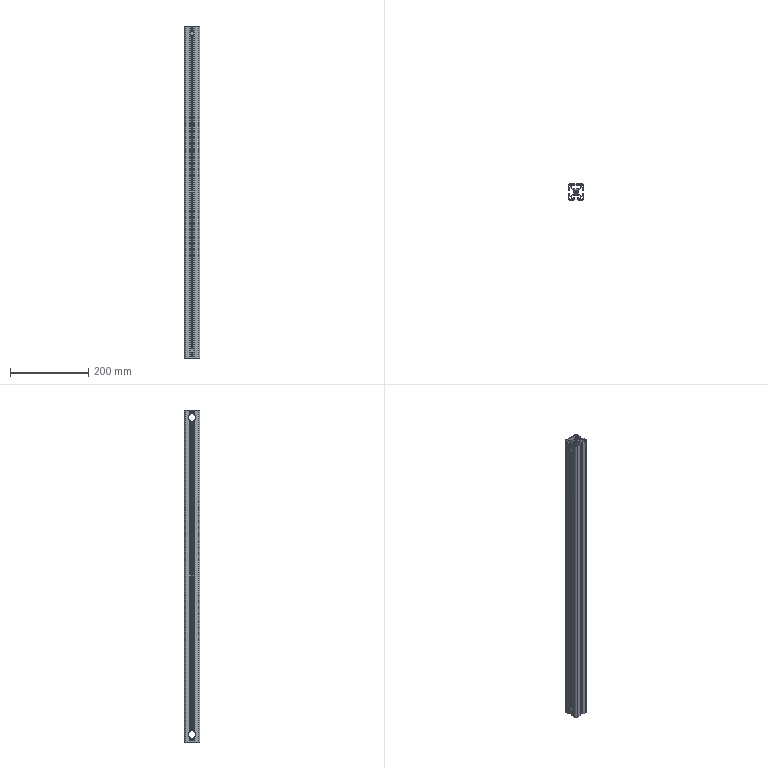Part | SolidWorks | features BaseBody 1, HoleWzd 1, MoveFace 1 | 1 solid | 242 faces | box 40 x 40 x 846 mm | volume 492509 mm3 | plane 187 | cylinder 55 | commonest cylinder face diameters 6.8 x15 2 x14 19 x12 1 x6 5 x4 9 x4